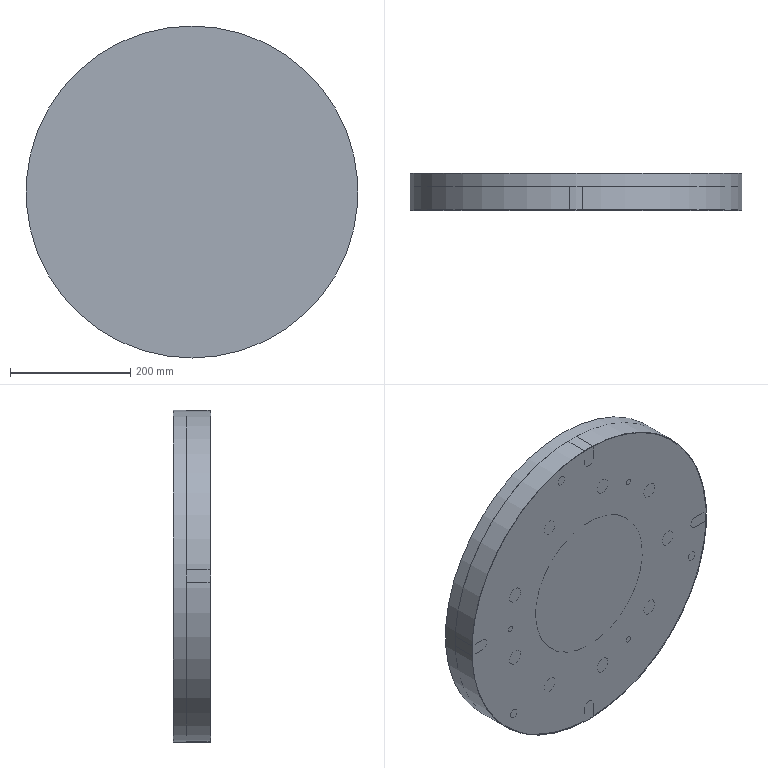NC program | NX | posted with a generic post | part box 552 x 62 x 552 mm
Whole program:
N10 G17 G21 G94 G90
(点窝 , TOOL : 点窝)
N12 T01 M6
N14 G54
N16 G17 G0 G90 X241.481 Y64.705 S0 M3
N18 G43 Z19. H1
N20 G94 G82 G99 Z-26. F80. P200 R8.
N22 G80
N24 G0 Z23.
N26 G82 X141.718 Y118.916 Z-11. F80. P200 R23.
N28 X92.5 Y160.215
N30 X32.125 Y182.189
N32 X-92.5 Y160.215
N34 X-176.777 Y176.777 Z-26. R8.
N36 G80
N38 G0 Z23.
N40 G82 X-173.843 Y63.274 Z-11. F80. P200 R23.
N42 X-185. Y0.
N44 X-173.843 Y-63.274
N46 X-92.5 Y-160.215
N48 X-64.705 Y-241.481 Z-26. R8.
N50 G80
N52 G0 Z23.
N54 G82 X32.125 Y-182.189 Z-11. F80. P200 R23.
N56 X92.5 Y-160.215
N58 X141.718 Y-118.916
N60 X185. Y0.
N62 G80
N64 G0 X185. Y0. Z19.
N66 M5
(DRILLING , TOOL : D9)
N68 T00 M6
N70 G54
N72 G17 G0 G90 X185. Y0. S900 M3
N74 G43 Z19. H0
N76 G94 G83 G99 Z-69.704 F80. Q4. R8.
N78 G0 Z-6.
N80 G83 X141.718 Y118.916 Z-69.704 Q4. R8.
N82 G0 Z-6.
N84 G83 X32.125 Y182.189 Z-69.704 Q4. R8.
N86 G0 Z-6.
N88 G83 X-92.5 Y160.215 Z-69.704 Q4. R8.
N90 G0 Z-6.
N92 G83 X-173.843 Y63.274 Z-69.704 Q4. R8.
N94 G0 Z-6.
N96 G83 Y-63.274 Z-69.704 Q4. R8.
N98 G0 Z-6.
N100 G83 X-92.5 Y-160.215 Z-69.704 Q4. R8.
N102 G0 Z-6.
N104 G83 X32.125 Y-182.189 Z-69.704 Q4. R8.
N106 G0 Z-6.
N108 G83 X141.718 Y-118.916 Z-69.704 Q4. R8.
N110 G0 Z-6.
N112 G80
N114 G0 X141.718 Y-118.916 Z19.
N116 M5
N118 M2